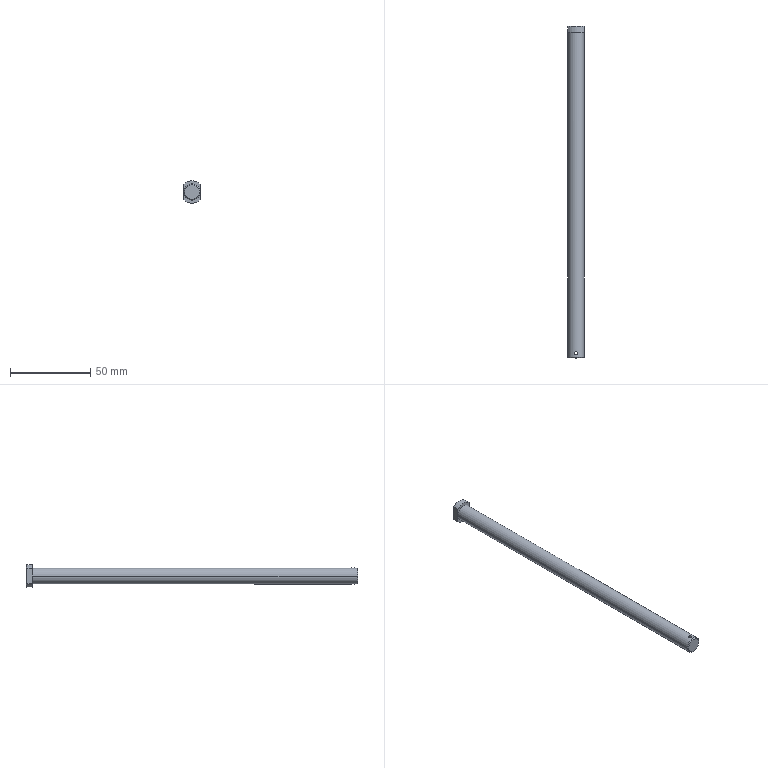Part | SolidWorks | features ICE 3, Chamfer 1, Revolution 1 | 1 solid | 16 faces | box 10 x 207 x 14 mm | volume 16414 mm3 | cylinder 6 | plane 6 | cone 4 | commonest cylinder face diameters 2 x2 10 x2 14 x2
STEP:
#1=CARTESIAN_POINT('',(1.,-204.,-4.899));
#2=VERTEX_POINT('',#1);
#3=CARTESIAN_POINT('',(-1.,-204.,-4.899));
#4=VERTEX_POINT('',#3);
#5=CARTESIAN_POINT('',(1.,-204.,-4.899));
#6=CARTESIAN_POINT('',(1.,-204.133,-4.899));
#7=CARTESIAN_POINT('',(0.9738,-204.263,-4.905));
#8=CARTESIAN_POINT('',(0.8733,-204.505,-4.923));
#9=CARTESIAN_POINT('',(0.799,-204.615,-4.937));
#10=CARTESIAN_POINT('',(0.6149,-204.799,-4.963));
#11=CARTESIAN_POINT('',(0.5036,-204.874,-4.976));
#12=CARTESIAN_POINT('',(0.2631,-204.974,-4.995));
#13=CARTESIAN_POINT('',(0.1312,-205.,-5.));
#14=CARTESIAN_POINT('',(-0.1304,-205.,-5.));
#15=CARTESIAN_POINT('',(-0.2616,-204.974,-4.995));
#16=CARTESIAN_POINT('',(-0.5042,-204.873,-4.976));
#17=CARTESIAN_POINT('',(-0.6142,-204.8,-4.963));
#18=CARTESIAN_POINT('',(-0.8001,-204.614,-4.936));
#19=CARTESIAN_POINT('',(-0.8736,-204.504,-4.923));
#20=CARTESIAN_POINT('',(-0.9739,-204.262,-4.905));
#21=CARTESIAN_POINT('',(-1.,-204.131,-4.899));
#22=CARTESIAN_POINT('',(-1.,-204.,-4.899));
#23=B_SPLINE_CURVE_WITH_KNOTS('',3,(#5,#6,#7,#8,#9,#10,#11,#12,#13,#14,#15,#16,#17,#18,#19,#20,#21,#22),.UNSPECIFIED.,.F.,.F.,(4,2,2,2,2,2,2,2,4),(0.,0.0003918,0.0007836,0.001175,0.001567,0.001959,0.002351,0.002743,0.003134),.UNSPECIFIED.);
#24=EDGE_CURVE('',#2,#4,#23,.T.);
#25=ORIENTED_EDGE('',*,*,#24,.T.);
#26=CARTESIAN_POINT('',(-1.,-204.,4.899));
#27=VERTEX_POINT('',#26);
#28=CARTESIAN_POINT('',(-1.,-204.,-7.));
#29=DIRECTION('',(0.,0.,1.));
#30=VECTOR('',#29,1000.);
#31=LINE('',#28,#30);
#32=EDGE_CURVE('',#4,#27,#31,.T.);
#33=ORIENTED_EDGE('',*,*,#32,.T.);
#34=CARTESIAN_POINT('',(1.,-204.,4.899));
#35=VERTEX_POINT('',#34);
#36=CARTESIAN_POINT('',(-1.,-204.,4.899));
#37=CARTESIAN_POINT('',(-1.,-204.131,4.899));
#38=CARTESIAN_POINT('',(-0.9737,-204.263,4.905));
#39=CARTESIAN_POINT('',(-0.8739,-204.503,4.923));
#40=CARTESIAN_POINT('',(-0.7996,-204.614,4.937));
#41=CARTESIAN_POINT('',(-0.6154,-204.799,4.963));
#42=CARTESIAN_POINT('',(-0.5052,-204.873,4.976));
#43=CARTESIAN_POINT('',(-0.2626,-204.974,4.995));
#44=CARTESIAN_POINT('',(-0.1325,-205.,5.));
#45=CARTESIAN_POINT('',(0.1315,-205.,5.));
#46=CARTESIAN_POINT('',(0.2621,-204.974,4.995));
#47=CARTESIAN_POINT('',(0.5037,-204.874,4.976));
#48=CARTESIAN_POINT('',(0.6147,-204.799,4.963));
#49=CARTESIAN_POINT('',(0.7986,-204.616,4.937));
#50=CARTESIAN_POINT('',(0.8732,-204.504,4.923));
#51=CARTESIAN_POINT('',(0.9733,-204.264,4.905));
#52=CARTESIAN_POINT('',(1.,-204.132,4.899));
#53=CARTESIAN_POINT('',(1.,-204.,4.899));
#54=B_SPLINE_CURVE_WITH_KNOTS('',3,(#36,#37,#38,#39,#40,#41,#42,#43,#44,#45,#46,#47,#48,#49,#50,#51,#52,#53),.UNSPECIFIED.,.F.,.F.,(4,2,2,2,2,2,2,2,4),(0.003134,0.003526,0.003918,0.004309,0.004701,0.005093,0.005485,0.005876,0.006268),.UNSPECIFIED.);
#55=EDGE_CURVE('',#27,#35,#54,.T.);
#56=ORIENTED_EDGE('',*,*,#55,.T.);
#57=CARTESIAN_POINT('',(1.,-204.,-7.));
#58=DIRECTION('',(0.,0.,1.));
#59=VECTOR('',#58,1000.);
#60=LINE('',#57,#59);
#61=EDGE_CURVE('',#2,#35,#60,.T.);
#62=ORIENTED_EDGE('',*,*,#61,.F.);
#63=EDGE_LOOP('',(#25,#33,#56,#62));
#64=FACE_OUTER_BOUND('',#63,.T.);
#65=CARTESIAN_POINT('',(0.,-204.,-7.));
#66=DIRECTION('',(0.,0.,1.));
#67=DIRECTION('',(1.,0.,0.));
#68=AXIS2_PLACEMENT_3D('',#65,#66,#67);
#69=CYLINDRICAL_SURFACE('',#68,1.);
#70=ADVANCED_FACE('',(#64),#69,.F.);
#71=CARTESIAN_POINT('',(4.5,-207.,0.));
#72=VERTEX_POINT('',#71);
#73=CARTESIAN_POINT('',(-4.5,-207.,0.));
#74=VERTEX_POINT('',#73);
#75=CARTESIAN_POINT('',(0.,-207.,0.));
#76=DIRECTION('',(0.,-1.,0.));
#77=DIRECTION('',(1.,0.,0.));
#78=AXIS2_PLACEMENT_3D('',#75,#76,#77);
#79=CIRCLE('',#78,4.5);
#80=EDGE_CURVE('',#72,#74,#79,.T.);
#81=ORIENTED_EDGE('',*,*,#80,.F.);
#82=CARTESIAN_POINT('',(5.,-206.5,0.));
#83=VERTEX_POINT('',#82);
#84=CARTESIAN_POINT('',(4.5,-207.,0.));
#85=DIRECTION('',(0.7071,0.7071,0.));
#86=VECTOR('',#85,1000.);
#87=LINE('',#84,#86);
#88=EDGE_CURVE('',#72,#83,#87,.T.);
#89=ORIENTED_EDGE('',*,*,#88,.T.);
#90=CARTESIAN_POINT('',(-5.,-206.5,0.));
#91=VERTEX_POINT('',#90);
#92=CARTESIAN_POINT('',(0.,-206.5,0.));
#93=DIRECTION('',(0.,1.,0.));
#94=DIRECTION('',(1.,0.,0.));
#95=AXIS2_PLACEMENT_3D('',#92,#93,#94);
#96=CIRCLE('',#95,5.);
#97=EDGE_CURVE('',#91,#83,#96,.T.);
#98=ORIENTED_EDGE('',*,*,#97,.F.);
#99=CARTESIAN_POINT('',(-4.5,-207.,0.));
#100=DIRECTION('',(-0.7071,0.7071,0.));
#101=VECTOR('',#100,1000.);
#102=LINE('',#99,#101);
#103=EDGE_CURVE('',#74,#91,#102,.T.);
#104=ORIENTED_EDGE('',*,*,#103,.F.);
#105=EDGE_LOOP('',(#81,#89,#98,#104));
#106=FACE_OUTER_BOUND('',#105,.T.);
#107=CARTESIAN_POINT('',(0.,-207.,0.));
#108=DIRECTION('',(0.,1.,0.));
#109=DIRECTION('',(-1.,0.,0.));
#110=AXIS2_PLACEMENT_3D('',#107,#108,#109);
#111=CONICAL_SURFACE('',#110,4.5,0.7854);
#112=ADVANCED_FACE('',(#106),#111,.T.);
#113=CARTESIAN_POINT('',(1.,-204.,4.899));
#114=CARTESIAN_POINT('',(1.,-203.867,4.899));
#115=CARTESIAN_POINT('',(0.9738,-203.737,4.905));
#116=CARTESIAN_POINT('',(0.8733,-203.495,4.923));
#117=CARTESIAN_POINT('',(0.799,-203.385,4.937));
#118=CARTESIAN_POINT('',(0.6149,-203.201,4.963));
#119=CARTESIAN_POINT('',(0.5036,-203.126,4.976));
#120=CARTESIAN_POINT('',(0.2631,-203.026,4.995));
#121=CARTESIAN_POINT('',(0.1312,-203.,5.));
#122=CARTESIAN_POINT('',(-0.1304,-203.,5.));
#123=CARTESIAN_POINT('',(-0.2616,-203.026,4.995));
#124=CARTESIAN_POINT('',(-0.5042,-203.127,4.976));
#125=CARTESIAN_POINT('',(-0.6142,-203.2,4.963));
#126=CARTESIAN_POINT('',(-0.8001,-203.386,4.936));
#127=CARTESIAN_POINT('',(-0.8736,-203.496,4.923));
#128=CARTESIAN_POINT('',(-0.9739,-203.738,4.905));
#129=CARTESIAN_POINT('',(-1.,-203.869,4.899));
#130=CARTESIAN_POINT('',(-1.,-204.,4.899));
#131=B_SPLINE_CURVE_WITH_KNOTS('',3,(#113,#114,#115,#116,#117,#118,#119,#120,#121,#122,#123,#124,#125,#126,#127,#128,#129,#130),.UNSPECIFIED.,.F.,.F.,(4,2,2,2,2,2,2,2,4),(0.,0.0003918,0.0007836,0.001175,0.001567,0.001959,0.002351,0.002743,0.003134),.UNSPECIFIED.);
#132=EDGE_CURVE('',#35,#27,#131,.T.);
#133=ORIENTED_EDGE('',*,*,#132,.F.);
#134=ORIENTED_EDGE('',*,*,#55,.F.);
#135=EDGE_LOOP('',(#133,#134));
#136=FACE_BOUND('',#135,.T.);
#137=CARTESIAN_POINT('',(5.,-4.,0.));
#138=VERTEX_POINT('',#137);
#139=CARTESIAN_POINT('',(-5.,-4.,0.));
#140=VERTEX_POINT('',#139);
#141=CARTESIAN_POINT('',(0.,-4.,0.));
#142=DIRECTION('',(0.,-1.,0.));
#143=DIRECTION('',(1.,0.,0.));
#144=AXIS2_PLACEMENT_3D('',#141,#142,#143);
#145=CIRCLE('',#144,5.);
#146=EDGE_CURVE('',#138,#140,#145,.T.);
#147=ORIENTED_EDGE('',*,*,#146,.T.);
#148=CARTESIAN_POINT('',(-5.,-318.988,0.));
#149=DIRECTION('',(0.,-1.,0.));
#150=VECTOR('',#149,1000.);
#151=LINE('',#148,#150);
#152=EDGE_CURVE('',#140,#91,#151,.T.);
#153=ORIENTED_EDGE('',*,*,#152,.T.);
#154=ORIENTED_EDGE('',*,*,#97,.T.);
#155=CARTESIAN_POINT('',(5.,-318.988,0.));
#156=DIRECTION('',(0.,-1.,0.));
#157=VECTOR('',#156,1000.);
#158=LINE('',#155,#157);
#159=EDGE_CURVE('',#138,#83,#158,.T.);
#160=ORIENTED_EDGE('',*,*,#159,.F.);
#161=EDGE_LOOP('',(#147,#153,#154,#160));
#162=FACE_OUTER_BOUND('',#161,.T.);
#163=CARTESIAN_POINT('',(0.,-318.988,0.));
#164=DIRECTION('',(0.,-1.,0.));
#165=DIRECTION('',(1.,0.,0.));
#166=AXIS2_PLACEMENT_3D('',#163,#164,#165);
#167=CYLINDRICAL_SURFACE('',#166,5.);
#168=ADVANCED_FACE('',(#136,#162),#167,.T.);
#169=CARTESIAN_POINT('',(5.,-4.,-4.899));
#170=VERTEX_POINT('',#169);
#171=CARTESIAN_POINT('',(5.,-0.5,-4.899));
#172=VERTEX_POINT('',#171);
#173=CARTESIAN_POINT('',(5.,-318.988,-4.899));
#174=DIRECTION('',(0.,1.,0.));
#175=VECTOR('',#174,1000.);
#176=LINE('',#173,#175);
#177=EDGE_CURVE('',#170,#172,#176,.T.);
#178=ORIENTED_EDGE('',*,*,#177,.F.);
#179=CARTESIAN_POINT('',(-5.,-4.,-4.899));
#180=VERTEX_POINT('',#179);
#181=CARTESIAN_POINT('',(0.,-4.,0.));
#182=DIRECTION('',(0.,-1.,0.));
#183=DIRECTION('',(1.,0.,0.));
#184=AXIS2_PLACEMENT_3D('',#181,#182,#183);
#185=CIRCLE('',#184,7.);
#186=EDGE_CURVE('',#180,#170,#185,.T.);
#187=ORIENTED_EDGE('',*,*,#186,.F.);
#188=CARTESIAN_POINT('',(-5.,-0.5,-4.899));
#189=VERTEX_POINT('',#188);
#190=CARTESIAN_POINT('',(-5.,-318.988,-4.899));
#191=DIRECTION('',(0.,-1.,0.));
#192=VECTOR('',#191,1000.);
#193=LINE('',#190,#192);
#194=EDGE_CURVE('',#189,#180,#193,.T.);
#195=ORIENTED_EDGE('',*,*,#194,.F.);
#196=CARTESIAN_POINT('',(0.,-0.5,0.));
#197=DIRECTION('',(0.,-1.,0.));
#198=DIRECTION('',(-1.,0.,0.));
#199=AXIS2_PLACEMENT_3D('',#196,#197,#198);
#200=CIRCLE('',#199,7.);
#201=EDGE_CURVE('',#189,#172,#200,.T.);
#202=ORIENTED_EDGE('',*,*,#201,.T.);
#203=EDGE_LOOP('',(#178,#187,#195,#202));
#204=FACE_OUTER_BOUND('',#203,.T.);
#205=CARTESIAN_POINT('',(0.,-318.988,0.));
#206=DIRECTION('',(0.,-1.,0.));
#207=DIRECTION('',(1.,0.,0.));
#208=AXIS2_PLACEMENT_3D('',#205,#206,#207);
#209=CYLINDRICAL_SURFACE('',#208,7.);
#210=ADVANCED_FACE('',(#204),#209,.T.);
#211=CARTESIAN_POINT('',(5.,-4.,4.899));
#212=VERTEX_POINT('',#211);
#213=CARTESIAN_POINT('',(5.,-4.,-7.));
#214=DIRECTION('',(0.,0.,1.));
#215=VECTOR('',#214,1000.);
#216=LINE('',#213,#215);
#217=EDGE_CURVE('',#138,#212,#216,.T.);
#218=ORIENTED_EDGE('',*,*,#217,.T.);
#219=CARTESIAN_POINT('',(-5.,-4.,4.899));
#220=VERTEX_POINT('',#219);
#221=CARTESIAN_POINT('',(0.,-4.,0.));
#222=DIRECTION('',(0.,-1.,0.));
#223=DIRECTION('',(1.,0.,0.));
#224=AXIS2_PLACEMENT_3D('',#221,#222,#223);
#225=CIRCLE('',#224,7.);
#226=EDGE_CURVE('',#212,#220,#225,.T.);
#227=ORIENTED_EDGE('',*,*,#226,.T.);
#228=CARTESIAN_POINT('',(-5.,-4.,-7.));
#229=DIRECTION('',(0.,0.,1.));
#230=VECTOR('',#229,1000.);
#231=LINE('',#228,#230);
#232=EDGE_CURVE('',#140,#220,#231,.T.);
#233=ORIENTED_EDGE('',*,*,#232,.F.);
#234=ORIENTED_EDGE('',*,*,#146,.F.);
#235=EDGE_LOOP('',(#218,#227,#233,#234));
#236=FACE_OUTER_BOUND('',#235,.T.);
#237=CARTESIAN_POINT('',(7.,-4.,0.));
#238=DIRECTION('',(0.,-1.,0.));
#239=DIRECTION('',(1.,0.,0.));
#240=AXIS2_PLACEMENT_3D('',#237,#238,#239);
#241=PLANE('',#240);
#242=ADVANCED_FACE('',(#236),#241,.T.);
#243=CARTESIAN_POINT('',(5.,0.,-4.153));
#244=VERTEX_POINT('',#243);
#245=CARTESIAN_POINT('',(5.,-0.5,-4.899));
#246=CARTESIAN_POINT('',(5.,-0.3284,-4.654));
#247=CARTESIAN_POINT('',(5.,-0.1612,-4.406));
#248=CARTESIAN_POINT('',(5.,0.,-4.153));
#249=B_SPLINE_CURVE_WITH_KNOTS('',3,(#245,#246,#247,#248),.UNSPECIFIED.,.F.,.F.,(4,4),(0.01284,0.01374),.UNSPECIFIED.);
#250=EDGE_CURVE('',#172,#244,#249,.T.);
#251=ORIENTED_EDGE('',*,*,#250,.F.);
#252=ORIENTED_EDGE('',*,*,#201,.F.);
#253=CARTESIAN_POINT('',(-5.,0.,-4.153));
#254=VERTEX_POINT('',#253);
#255=CARTESIAN_POINT('',(-5.,0.,-4.153));
#256=CARTESIAN_POINT('',(-5.,-0.1613,-4.406));
#257=CARTESIAN_POINT('',(-5.,-0.3287,-4.654));
#258=CARTESIAN_POINT('',(-5.,-0.5,-4.899));
#259=B_SPLINE_CURVE_WITH_KNOTS('',3,(#255,#256,#257,#258),.UNSPECIFIED.,.F.,.F.,(4,4),(0.02258,0.02346),.UNSPECIFIED.);
#260=EDGE_CURVE('',#254,#189,#259,.T.);
#261=ORIENTED_EDGE('',*,*,#260,.F.);
#262=CARTESIAN_POINT('',(0.,0.,0.));
#263=DIRECTION('',(0.,1.,0.));
#264=DIRECTION('',(-1.,0.,0.));
#265=AXIS2_PLACEMENT_3D('',#262,#263,#264);
#266=CIRCLE('',#265,6.5);
#267=EDGE_CURVE('',#244,#254,#266,.T.);
#268=ORIENTED_EDGE('',*,*,#267,.F.);
#269=EDGE_LOOP('',(#251,#252,#261,#268));
#270=FACE_OUTER_BOUND('',#269,.T.);
#271=CARTESIAN_POINT('',(0.,-0.5,0.));
#272=DIRECTION('',(0.,-1.,0.));
#273=DIRECTION('',(1.,0.,0.));
#274=AXIS2_PLACEMENT_3D('',#271,#272,#273);
#275=CONICAL_SURFACE('',#274,7.,0.7854);
#276=ADVANCED_FACE('',(#270),#275,.T.);
#277=CARTESIAN_POINT('',(5.,0.,4.153));
#278=VERTEX_POINT('',#277);
#279=CARTESIAN_POINT('',(5.,0.,-7.));
#280=DIRECTION('',(0.,0.,1.));
#281=VECTOR('',#280,1000.);
#282=LINE('',#279,#281);
#283=EDGE_CURVE('',#244,#278,#282,.T.);
#284=ORIENTED_EDGE('',*,*,#283,.F.);
#285=ORIENTED_EDGE('',*,*,#267,.T.);
#286=CARTESIAN_POINT('',(-5.,0.,4.153));
#287=VERTEX_POINT('',#286);
#288=CARTESIAN_POINT('',(-5.,0.,-7.));
#289=DIRECTION('',(0.,0.,1.));
#290=VECTOR('',#289,1000.);
#291=LINE('',#288,#290);
#292=EDGE_CURVE('',#254,#287,#291,.T.);
#293=ORIENTED_EDGE('',*,*,#292,.T.);
#294=CARTESIAN_POINT('',(0.,0.,0.));
#295=DIRECTION('',(0.,1.,0.));
#296=DIRECTION('',(-1.,0.,0.));
#297=AXIS2_PLACEMENT_3D('',#294,#295,#296);
#298=CIRCLE('',#297,6.5);
#299=EDGE_CURVE('',#287,#278,#298,.T.);
#300=ORIENTED_EDGE('',*,*,#299,.T.);
#301=EDGE_LOOP('',(#284,#285,#293,#300));
#302=FACE_OUTER_BOUND('',#301,.T.);
#303=CARTESIAN_POINT('',(0.,0.,0.));
#304=DIRECTION('',(0.,1.,0.));
#305=DIRECTION('',(-1.,0.,0.));
#306=AXIS2_PLACEMENT_3D('',#303,#304,#305);
#307=PLANE('',#306);
#308=ADVANCED_FACE('',(#302),#307,.T.);
#309=CARTESIAN_POINT('',(5.,-0.5,4.899));
#310=VERTEX_POINT('',#309);
#311=CARTESIAN_POINT('',(5.,-318.988,4.899));
#312=DIRECTION('',(0.,-1.,0.));
#313=VECTOR('',#312,1000.);
#314=LINE('',#311,#313);
#315=EDGE_CURVE('',#310,#212,#314,.T.);
#316=ORIENTED_EDGE('',*,*,#315,.F.);
#317=CARTESIAN_POINT('',(-5.,-0.5,4.899));
#318=VERTEX_POINT('',#317);
#319=CARTESIAN_POINT('',(0.,-0.5,0.));
#320=DIRECTION('',(0.,-1.,0.));
#321=DIRECTION('',(-1.,0.,0.));
#322=AXIS2_PLACEMENT_3D('',#319,#320,#321);
#323=CIRCLE('',#322,7.);
#324=EDGE_CURVE('',#310,#318,#323,.T.);
#325=ORIENTED_EDGE('',*,*,#324,.T.);
#326=CARTESIAN_POINT('',(-5.,-318.988,4.899));
#327=DIRECTION('',(0.,1.,0.));
#328=VECTOR('',#327,1000.);
#329=LINE('',#326,#328);
#330=EDGE_CURVE('',#220,#318,#329,.T.);
#331=ORIENTED_EDGE('',*,*,#330,.F.);
#332=ORIENTED_EDGE('',*,*,#226,.F.);
#333=EDGE_LOOP('',(#316,#325,#331,#332));
#334=FACE_OUTER_BOUND('',#333,.T.);
#335=CARTESIAN_POINT('',(0.,-318.988,0.));
#336=DIRECTION('',(0.,-1.,0.));
#337=DIRECTION('',(1.,0.,0.));
#338=AXIS2_PLACEMENT_3D('',#335,#336,#337);
#339=CYLINDRICAL_SURFACE('',#338,7.);
#340=ADVANCED_FACE('',(#334),#339,.T.);
#341=CARTESIAN_POINT('',(5.,-4.,-7.));
#342=DIRECTION('',(0.,0.,1.));
#343=VECTOR('',#342,1000.);
#344=LINE('',#341,#343);
#345=EDGE_CURVE('',#170,#138,#344,.T.);
#346=ORIENTED_EDGE('',*,*,#345,.T.);
#347=CARTESIAN_POINT('',(0.,-4.,0.));
#348=DIRECTION('',(0.,-1.,0.));
#349=DIRECTION('',(1.,0.,0.));
#350=AXIS2_PLACEMENT_3D('',#347,#348,#349);
#351=CIRCLE('',#350,5.);
#352=EDGE_CURVE('',#140,#138,#351,.T.);
#353=ORIENTED_EDGE('',*,*,#352,.F.);
#354=CARTESIAN_POINT('',(-5.,-4.,-7.));
#355=DIRECTION('',(0.,0.,1.));
#356=VECTOR('',#355,1000.);
#357=LINE('',#354,#356);
#358=EDGE_CURVE('',#180,#140,#357,.T.);
#359=ORIENTED_EDGE('',*,*,#358,.F.);
#360=ORIENTED_EDGE('',*,*,#186,.T.);
#361=EDGE_LOOP('',(#346,#353,#359,#360));
#362=FACE_OUTER_BOUND('',#361,.T.);
#363=CARTESIAN_POINT('',(7.,-4.,0.));
#364=DIRECTION('',(0.,-1.,0.));
#365=DIRECTION('',(1.,0.,0.));
#366=AXIS2_PLACEMENT_3D('',#363,#364,#365);
#367=PLANE('',#366);
#368=ADVANCED_FACE('',(#362),#367,.T.);
#369=ORIENTED_EDGE('',*,*,#152,.F.);
#370=ORIENTED_EDGE('',*,*,#352,.T.);
#371=ORIENTED_EDGE('',*,*,#159,.T.);
#372=CARTESIAN_POINT('',(0.,-206.5,0.));
#373=DIRECTION('',(0.,1.,0.));
#374=DIRECTION('',(1.,0.,0.));
#375=AXIS2_PLACEMENT_3D('',#372,#373,#374);
#376=CIRCLE('',#375,5.);
#377=EDGE_CURVE('',#83,#91,#376,.T.);
#378=ORIENTED_EDGE('',*,*,#377,.T.);
#379=EDGE_LOOP('',(#369,#370,#371,#378));
#380=FACE_OUTER_BOUND('',#379,.T.);
#381=ORIENTED_EDGE('',*,*,#24,.F.);
#382=CARTESIAN_POINT('',(-1.,-204.,-4.899));
#383=CARTESIAN_POINT('',(-1.,-203.869,-4.899));
#384=CARTESIAN_POINT('',(-0.9737,-203.737,-4.905));
#385=CARTESIAN_POINT('',(-0.8739,-203.497,-4.923));
#386=CARTESIAN_POINT('',(-0.7996,-203.386,-4.937));
#387=CARTESIAN_POINT('',(-0.6154,-203.201,-4.963));
#388=CARTESIAN_POINT('',(-0.5052,-203.127,-4.976));
#389=CARTESIAN_POINT('',(-0.2626,-203.026,-4.995));
#390=CARTESIAN_POINT('',(-0.1325,-203.,-5.));
#391=CARTESIAN_POINT('',(0.1315,-203.,-5.));
#392=CARTESIAN_POINT('',(0.2621,-203.026,-4.995));
#393=CARTESIAN_POINT('',(0.5037,-203.126,-4.976));
#394=CARTESIAN_POINT('',(0.6147,-203.201,-4.963));
#395=CARTESIAN_POINT('',(0.7986,-203.384,-4.937));
#396=CARTESIAN_POINT('',(0.8732,-203.496,-4.923));
#397=CARTESIAN_POINT('',(0.9733,-203.736,-4.905));
#398=CARTESIAN_POINT('',(1.,-203.868,-4.899));
#399=CARTESIAN_POINT('',(1.,-204.,-4.899));
#400=B_SPLINE_CURVE_WITH_KNOTS('',3,(#382,#383,#384,#385,#386,#387,#388,#389,#390,#391,#392,#393,#394,#395,#396,#397,#398,#399),.UNSPECIFIED.,.F.,.F.,(4,2,2,2,2,2,2,2,4),(0.003134,0.003526,0.003918,0.004309,0.004701,0.005093,0.005485,0.005876,0.006268),.UNSPECIFIED.);
#401=EDGE_CURVE('',#4,#2,#400,.T.);
#402=ORIENTED_EDGE('',*,*,#401,.F.);
#403=EDGE_LOOP('',(#381,#402));
#404=FACE_BOUND('',#403,.T.);
#405=CARTESIAN_POINT('',(0.,-318.988,0.));
#406=DIRECTION('',(0.,-1.,0.));
#407=DIRECTION('',(1.,0.,0.));
#408=AXIS2_PLACEMENT_3D('',#405,#406,#407);
#409=CYLINDRICAL_SURFACE('',#408,5.);
#410=ADVANCED_FACE('',(#380,#404),#409,.T.);
#411=CARTESIAN_POINT('',(0.,-207.,0.));
#412=DIRECTION('',(0.,-1.,0.));
#413=DIRECTION('',(1.,0.,0.));
#414=AXIS2_PLACEMENT_3D('',#411,#412,#413);
#415=CIRCLE('',#414,4.5);
#416=EDGE_CURVE('',#74,#72,#415,.T.);
#417=ORIENTED_EDGE('',*,*,#416,.T.);
#418=ORIENTED_EDGE('',*,*,#80,.T.);
#419=EDGE_LOOP('',(#417,#418));
#420=FACE_OUTER_BOUND('',#419,.T.);
#421=CARTESIAN_POINT('',(5.,-207.,0.));
#422=DIRECTION('',(0.,-1.,0.));
#423=DIRECTION('',(1.,0.,0.));
#424=AXIS2_PLACEMENT_3D('',#421,#422,#423);
#425=PLANE('',#424);
#426=ADVANCED_FACE('',(#420),#425,.T.);
#427=ORIENTED_EDGE('',*,*,#88,.F.);
#428=ORIENTED_EDGE('',*,*,#416,.F.);
#429=ORIENTED_EDGE('',*,*,#103,.T.);
#430=ORIENTED_EDGE('',*,*,#377,.F.);
#431=EDGE_LOOP('',(#427,#428,#429,#430));
#432=FACE_OUTER_BOUND('',#431,.T.);
#433=CARTESIAN_POINT('',(0.,-207.,0.));
#434=DIRECTION('',(0.,1.,0.));
#435=DIRECTION('',(-1.,0.,0.));
#436=AXIS2_PLACEMENT_3D('',#433,#434,#435);
#437=CONICAL_SURFACE('',#436,4.5,0.7854);
#438=ADVANCED_FACE('',(#432),#437,.T.);
#439=CARTESIAN_POINT('',(5.,0.,4.153));
#440=CARTESIAN_POINT('',(5.,-0.1613,4.406));
#441=CARTESIAN_POINT('',(5.,-0.3287,4.654));
#442=CARTESIAN_POINT('',(5.,-0.5,4.899));
#443=B_SPLINE_CURVE_WITH_KNOTS('',3,(#439,#440,#441,#442),.UNSPECIFIED.,.F.,.F.,(4,4),(0.02258,0.02346),.UNSPECIFIED.);
#444=EDGE_CURVE('',#278,#310,#443,.T.);
#445=ORIENTED_EDGE('',*,*,#444,.F.);
#446=ORIENTED_EDGE('',*,*,#299,.F.);
#447=CARTESIAN_POINT('',(-5.,-0.5,4.899));
#448=CARTESIAN_POINT('',(-5.,-0.3284,4.654));
#449=CARTESIAN_POINT('',(-5.,-0.1612,4.406));
#450=CARTESIAN_POINT('',(-5.,0.,4.153));
#451=B_SPLINE_CURVE_WITH_KNOTS('',3,(#447,#448,#449,#450),.UNSPECIFIED.,.F.,.F.,(4,4),(0.01284,0.01374),.UNSPECIFIED.);
#452=EDGE_CURVE('',#318,#287,#451,.T.);
#453=ORIENTED_EDGE('',*,*,#452,.F.);
#454=ORIENTED_EDGE('',*,*,#324,.F.);
#455=EDGE_LOOP('',(#445,#446,#453,#454));
#456=FACE_OUTER_BOUND('',#455,.T.);
#457=CARTESIAN_POINT('',(0.,-0.5,0.));
#458=DIRECTION('',(0.,-1.,0.));
#459=DIRECTION('',(1.,0.,0.));
#460=AXIS2_PLACEMENT_3D('',#457,#458,#459);
#461=CONICAL_SURFACE('',#460,7.,0.7854);
#462=ADVANCED_FACE('',(#456),#461,.T.);
#463=ORIENTED_EDGE('',*,*,#32,.F.);
#464=ORIENTED_EDGE('',*,*,#401,.T.);
#465=ORIENTED_EDGE('',*,*,#61,.T.);
#466=ORIENTED_EDGE('',*,*,#132,.T.);
#467=EDGE_LOOP('',(#463,#464,#465,#466));
#468=FACE_OUTER_BOUND('',#467,.T.);
#469=CARTESIAN_POINT('',(0.,-204.,-7.));
#470=DIRECTION('',(0.,0.,1.));
#471=DIRECTION('',(1.,0.,0.));
#472=AXIS2_PLACEMENT_3D('',#469,#470,#471);
#473=CYLINDRICAL_SURFACE('',#472,1.);
#474=ADVANCED_FACE('',(#468),#473,.F.);
#475=ORIENTED_EDGE('',*,*,#330,.T.);
#476=ORIENTED_EDGE('',*,*,#452,.T.);
#477=ORIENTED_EDGE('',*,*,#292,.F.);
#478=ORIENTED_EDGE('',*,*,#260,.T.);
#479=ORIENTED_EDGE('',*,*,#194,.T.);
#480=ORIENTED_EDGE('',*,*,#358,.T.);
#481=ORIENTED_EDGE('',*,*,#232,.T.);
#482=EDGE_LOOP('',(#475,#476,#477,#478,#479,#480,#481));
#483=FACE_OUTER_BOUND('',#482,.T.);
#484=CARTESIAN_POINT('',(-5.,-4.,-7.));
#485=DIRECTION('',(1.,0.,0.));
#486=DIRECTION('',(0.,0.,-1.));
#487=AXIS2_PLACEMENT_3D('',#484,#485,#486);
#488=PLANE('',#487);
#489=ADVANCED_FACE('',(#483),#488,.F.);
#490=ORIENTED_EDGE('',*,*,#177,.T.);
#491=ORIENTED_EDGE('',*,*,#250,.T.);
#492=ORIENTED_EDGE('',*,*,#283,.T.);
#493=ORIENTED_EDGE('',*,*,#444,.T.);
#494=ORIENTED_EDGE('',*,*,#315,.T.);
#495=ORIENTED_EDGE('',*,*,#217,.F.);
#496=ORIENTED_EDGE('',*,*,#345,.F.);
#497=EDGE_LOOP('',(#490,#491,#492,#493,#494,#495,#496));
#498=FACE_OUTER_BOUND('',#497,.T.);
#499=CARTESIAN_POINT('',(5.,-4.,-7.));
#500=DIRECTION('',(-1.,0.,0.));
#501=DIRECTION('',(0.,0.,1.));
#502=AXIS2_PLACEMENT_3D('',#499,#500,#501);
#503=PLANE('',#502);
#504=ADVANCED_FACE('',(#498),#503,.F.);
#505=CLOSED_SHELL('',(#70,#112,#168,#210,#242,#276,#308,#340,#368,#410,#426,#438,#462,#474,#489,#504));
#506=MANIFOLD_SOLID_BREP('',#505);
#507=CARTESIAN_POINT('',(0.,0.,0.));
#508=DIRECTION('',(0.,0.,1.));
#509=DIRECTION('',(1.,0.,0.));
#510=AXIS2_PLACEMENT_3D('',#507,#508,#509);
#511=(LENGTH_UNIT()NAMED_UNIT(*)SI_UNIT(.MILLI.,.METRE.));
#512=UNCERTAINTY_MEASURE_WITH_UNIT(LENGTH_MEASURE(0.00001),#511,'','');
#513=(NAMED_UNIT(*)PLANE_ANGLE_UNIT()SI_UNIT($,.RADIAN.));
#514=(NAMED_UNIT(*)SI_UNIT($,.STERADIAN.)SOLID_ANGLE_UNIT());
#515=(GEOMETRIC_REPRESENTATION_CONTEXT(3)GLOBAL_UNCERTAINTY_ASSIGNED_CONTEXT((#512))GLOBAL_UNIT_ASSIGNED_CONTEXT((#511,#513,#514))REPRESENTATION_CONTEXT('',''));
#516=ADVANCED_BREP_SHAPE_REPRESENTATION('',(#506,#510),#515);